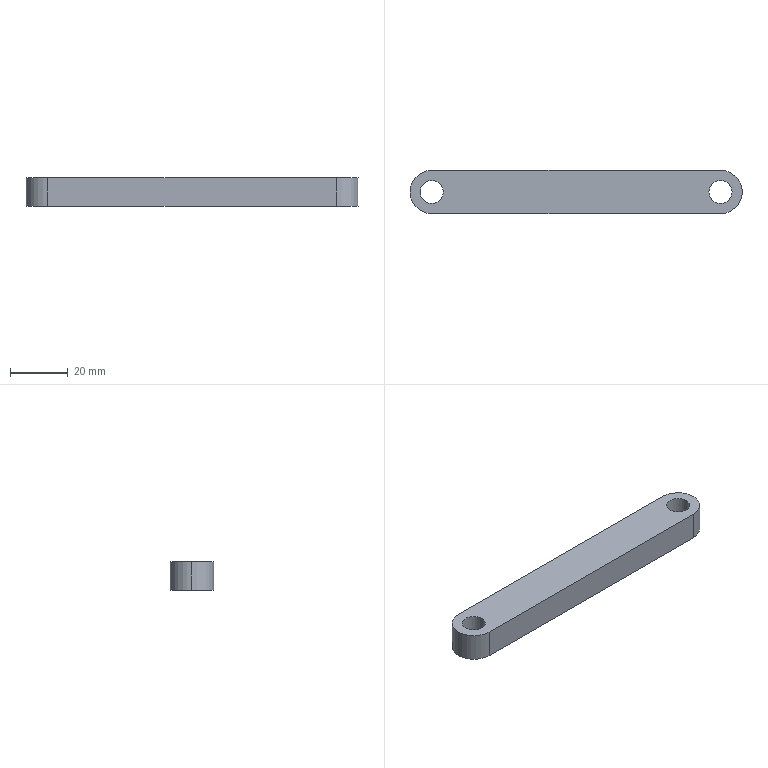Part | SolidWorks | features Extrusion 1 | 1 solid | 11 faces | box 115 x 15 x 10 mm | volume 15762 mm3 | cylinder 7 | plane 4 | commonest cylinder face diameters 8 x4 15 x3
STEP:
#1=CARTESIAN_POINT('',(96.,0.,10.));
#2=VERTEX_POINT('',#1);
#3=CARTESIAN_POINT('',(104.,0.,10.));
#4=VERTEX_POINT('',#3);
#5=CARTESIAN_POINT('',(100.,0.,10.));
#6=DIRECTION('',(0.,0.,1.));
#7=DIRECTION('',(1.,0.,0.));
#8=AXIS2_PLACEMENT_3D('',#5,#6,#7);
#9=CIRCLE('',#8,4.);
#10=EDGE_CURVE('',#2,#4,#9,.T.);
#11=ORIENTED_EDGE('',*,*,#10,.T.);
#12=CARTESIAN_POINT('',(104.,0.,0.));
#13=VERTEX_POINT('',#12);
#14=CARTESIAN_POINT('',(104.,0.,10.));
#15=DIRECTION('',(0.,0.,-1.));
#16=VECTOR('',#15,1000.);
#17=LINE('',#14,#16);
#18=EDGE_CURVE('',#4,#13,#17,.T.);
#19=ORIENTED_EDGE('',*,*,#18,.T.);
#20=CARTESIAN_POINT('',(96.,0.,0.));
#21=VERTEX_POINT('',#20);
#22=CARTESIAN_POINT('',(100.,0.,0.));
#23=DIRECTION('',(0.,0.,1.));
#24=DIRECTION('',(1.,0.,0.));
#25=AXIS2_PLACEMENT_3D('',#22,#23,#24);
#26=CIRCLE('',#25,4.);
#27=EDGE_CURVE('',#21,#13,#26,.T.);
#28=ORIENTED_EDGE('',*,*,#27,.F.);
#29=CARTESIAN_POINT('',(96.,0.,10.));
#30=DIRECTION('',(0.,0.,-1.));
#31=VECTOR('',#30,1000.);
#32=LINE('',#29,#31);
#33=EDGE_CURVE('',#2,#21,#32,.T.);
#34=ORIENTED_EDGE('',*,*,#33,.F.);
#35=EDGE_LOOP('',(#11,#19,#28,#34));
#36=FACE_OUTER_BOUND('',#35,.T.);
#37=CARTESIAN_POINT('',(100.,0.,10.));
#38=DIRECTION('',(0.,0.,-1.));
#39=DIRECTION('',(-1.,0.,0.));
#40=AXIS2_PLACEMENT_3D('',#37,#38,#39);
#41=CYLINDRICAL_SURFACE('',#40,4.);
#42=ADVANCED_FACE('',(#36),#41,.F.);
#43=CARTESIAN_POINT('',(-4.,0.,10.));
#44=VERTEX_POINT('',#43);
#45=CARTESIAN_POINT('',(4.,0.,10.));
#46=VERTEX_POINT('',#45);
#47=CARTESIAN_POINT('',(0.,0.,10.));
#48=DIRECTION('',(0.,0.,1.));
#49=DIRECTION('',(1.,0.,0.));
#50=AXIS2_PLACEMENT_3D('',#47,#48,#49);
#51=CIRCLE('',#50,4.);
#52=EDGE_CURVE('',#44,#46,#51,.T.);
#53=ORIENTED_EDGE('',*,*,#52,.T.);
#54=CARTESIAN_POINT('',(4.,0.,0.));
#55=VERTEX_POINT('',#54);
#56=CARTESIAN_POINT('',(4.,0.,10.));
#57=DIRECTION('',(0.,0.,-1.));
#58=VECTOR('',#57,1000.);
#59=LINE('',#56,#58);
#60=EDGE_CURVE('',#46,#55,#59,.T.);
#61=ORIENTED_EDGE('',*,*,#60,.T.);
#62=CARTESIAN_POINT('',(-4.,0.,0.));
#63=VERTEX_POINT('',#62);
#64=CARTESIAN_POINT('',(0.,0.,0.));
#65=DIRECTION('',(0.,0.,1.));
#66=DIRECTION('',(1.,0.,0.));
#67=AXIS2_PLACEMENT_3D('',#64,#65,#66);
#68=CIRCLE('',#67,4.);
#69=EDGE_CURVE('',#63,#55,#68,.T.);
#70=ORIENTED_EDGE('',*,*,#69,.F.);
#71=CARTESIAN_POINT('',(-4.,0.,10.));
#72=DIRECTION('',(0.,0.,-1.));
#73=VECTOR('',#72,1000.);
#74=LINE('',#71,#73);
#75=EDGE_CURVE('',#44,#63,#74,.T.);
#76=ORIENTED_EDGE('',*,*,#75,.F.);
#77=EDGE_LOOP('',(#53,#61,#70,#76));
#78=FACE_OUTER_BOUND('',#77,.T.);
#79=CARTESIAN_POINT('',(0.,0.,10.));
#80=DIRECTION('',(0.,0.,-1.));
#81=DIRECTION('',(-1.,0.,0.));
#82=AXIS2_PLACEMENT_3D('',#79,#80,#81);
#83=CYLINDRICAL_SURFACE('',#82,4.);
#84=ADVANCED_FACE('',(#78),#83,.F.);
#85=CARTESIAN_POINT('',(-7.5,0.,10.));
#86=VERTEX_POINT('',#85);
#87=CARTESIAN_POINT('',(0.,-7.5,10.));
#88=VERTEX_POINT('',#87);
#89=CARTESIAN_POINT('',(0.,0.,10.));
#90=DIRECTION('',(0.,0.,1.));
#91=DIRECTION('',(1.,0.,0.));
#92=AXIS2_PLACEMENT_3D('',#89,#90,#91);
#93=CIRCLE('',#92,7.5);
#94=EDGE_CURVE('',#86,#88,#93,.T.);
#95=ORIENTED_EDGE('',*,*,#94,.F.);
#96=CARTESIAN_POINT('',(-7.5,0.,0.));
#97=VERTEX_POINT('',#96);
#98=CARTESIAN_POINT('',(-7.5,0.,10.));
#99=DIRECTION('',(0.,0.,-1.));
#100=VECTOR('',#99,1000.);
#101=LINE('',#98,#100);
#102=EDGE_CURVE('',#86,#97,#101,.T.);
#103=ORIENTED_EDGE('',*,*,#102,.T.);
#104=CARTESIAN_POINT('',(0.,-7.5,0.));
#105=VERTEX_POINT('',#104);
#106=CARTESIAN_POINT('',(0.,0.,0.));
#107=DIRECTION('',(0.,0.,1.));
#108=DIRECTION('',(1.,0.,0.));
#109=AXIS2_PLACEMENT_3D('',#106,#107,#108);
#110=CIRCLE('',#109,7.5);
#111=EDGE_CURVE('',#97,#105,#110,.T.);
#112=ORIENTED_EDGE('',*,*,#111,.T.);
#113=CARTESIAN_POINT('',(0.,-7.5,10.));
#114=DIRECTION('',(0.,0.,-1.));
#115=VECTOR('',#114,1000.);
#116=LINE('',#113,#115);
#117=EDGE_CURVE('',#88,#105,#116,.T.);
#118=ORIENTED_EDGE('',*,*,#117,.F.);
#119=EDGE_LOOP('',(#95,#103,#112,#118));
#120=FACE_OUTER_BOUND('',#119,.T.);
#121=CARTESIAN_POINT('',(0.,0.,10.));
#122=DIRECTION('',(0.,0.,-1.));
#123=DIRECTION('',(-1.,0.,0.));
#124=AXIS2_PLACEMENT_3D('',#121,#122,#123);
#125=CYLINDRICAL_SURFACE('',#124,7.5);
#126=ADVANCED_FACE('',(#120),#125,.T.);
#127=ORIENTED_EDGE('',*,*,#52,.F.);
#128=CARTESIAN_POINT('',(0.,0.,10.));
#129=DIRECTION('',(0.,0.,1.));
#130=DIRECTION('',(1.,0.,0.));
#131=AXIS2_PLACEMENT_3D('',#128,#129,#130);
#132=CIRCLE('',#131,4.);
#133=EDGE_CURVE('',#46,#44,#132,.T.);
#134=ORIENTED_EDGE('',*,*,#133,.F.);
#135=EDGE_LOOP('',(#127,#134));
#136=FACE_BOUND('',#135,.T.);
#137=CARTESIAN_POINT('',(0.,7.5,10.));
#138=VERTEX_POINT('',#137);
#139=CARTESIAN_POINT('',(0.,0.,10.));
#140=DIRECTION('',(0.,0.,1.));
#141=DIRECTION('',(1.,0.,0.));
#142=AXIS2_PLACEMENT_3D('',#139,#140,#141);
#143=CIRCLE('',#142,7.5);
#144=EDGE_CURVE('',#138,#86,#143,.T.);
#145=ORIENTED_EDGE('',*,*,#144,.T.);
#146=ORIENTED_EDGE('',*,*,#94,.T.);
#147=CARTESIAN_POINT('',(100.,-7.5,10.));
#148=VERTEX_POINT('',#147);
#149=CARTESIAN_POINT('',(100.,-7.5,10.));
#150=DIRECTION('',(1.,0.,0.));
#151=VECTOR('',#150,1000.);
#152=LINE('',#149,#151);
#153=EDGE_CURVE('',#88,#148,#152,.T.);
#154=ORIENTED_EDGE('',*,*,#153,.T.);
#155=CARTESIAN_POINT('',(100.,7.5,10.));
#156=VERTEX_POINT('',#155);
#157=CARTESIAN_POINT('',(100.,0.,10.));
#158=DIRECTION('',(0.,0.,1.));
#159=DIRECTION('',(1.,0.,0.));
#160=AXIS2_PLACEMENT_3D('',#157,#158,#159);
#161=CIRCLE('',#160,7.5);
#162=EDGE_CURVE('',#148,#156,#161,.T.);
#163=ORIENTED_EDGE('',*,*,#162,.T.);
#164=CARTESIAN_POINT('',(0.,7.5,10.));
#165=DIRECTION('',(-1.,0.,0.));
#166=VECTOR('',#165,1000.);
#167=LINE('',#164,#166);
#168=EDGE_CURVE('',#156,#138,#167,.T.);
#169=ORIENTED_EDGE('',*,*,#168,.T.);
#170=EDGE_LOOP('',(#145,#146,#154,#163,#169));
#171=FACE_OUTER_BOUND('',#170,.T.);
#172=ORIENTED_EDGE('',*,*,#10,.F.);
#173=CARTESIAN_POINT('',(100.,0.,10.));
#174=DIRECTION('',(0.,0.,1.));
#175=DIRECTION('',(1.,0.,0.));
#176=AXIS2_PLACEMENT_3D('',#173,#174,#175);
#177=CIRCLE('',#176,4.);
#178=EDGE_CURVE('',#4,#2,#177,.T.);
#179=ORIENTED_EDGE('',*,*,#178,.F.);
#180=EDGE_LOOP('',(#172,#179));
#181=FACE_BOUND('',#180,.T.);
#182=CARTESIAN_POINT('',(0.,0.,10.));
#183=DIRECTION('',(0.,0.,1.));
#184=DIRECTION('',(1.,0.,0.));
#185=AXIS2_PLACEMENT_3D('',#182,#183,#184);
#186=PLANE('',#185);
#187=ADVANCED_FACE('',(#136,#171,#181),#186,.T.);
#188=CARTESIAN_POINT('',(0.,7.5,0.));
#189=VERTEX_POINT('',#188);
#190=CARTESIAN_POINT('',(0.,0.,0.));
#191=DIRECTION('',(0.,0.,1.));
#192=DIRECTION('',(1.,0.,0.));
#193=AXIS2_PLACEMENT_3D('',#190,#191,#192);
#194=CIRCLE('',#193,7.5);
#195=EDGE_CURVE('',#189,#97,#194,.T.);
#196=ORIENTED_EDGE('',*,*,#195,.F.);
#197=CARTESIAN_POINT('',(100.,7.5,0.));
#198=VERTEX_POINT('',#197);
#199=CARTESIAN_POINT('',(0.,7.5,0.));
#200=DIRECTION('',(-1.,0.,0.));
#201=VECTOR('',#200,1000.);
#202=LINE('',#199,#201);
#203=EDGE_CURVE('',#198,#189,#202,.T.);
#204=ORIENTED_EDGE('',*,*,#203,.F.);
#205=CARTESIAN_POINT('',(100.,-7.5,0.));
#206=VERTEX_POINT('',#205);
#207=CARTESIAN_POINT('',(100.,0.,0.));
#208=DIRECTION('',(0.,0.,1.));
#209=DIRECTION('',(1.,0.,0.));
#210=AXIS2_PLACEMENT_3D('',#207,#208,#209);
#211=CIRCLE('',#210,7.5);
#212=EDGE_CURVE('',#206,#198,#211,.T.);
#213=ORIENTED_EDGE('',*,*,#212,.F.);
#214=CARTESIAN_POINT('',(100.,-7.5,0.));
#215=DIRECTION('',(1.,0.,0.));
#216=VECTOR('',#215,1000.);
#217=LINE('',#214,#216);
#218=EDGE_CURVE('',#105,#206,#217,.T.);
#219=ORIENTED_EDGE('',*,*,#218,.F.);
#220=ORIENTED_EDGE('',*,*,#111,.F.);
#221=EDGE_LOOP('',(#196,#204,#213,#219,#220));
#222=FACE_OUTER_BOUND('',#221,.T.);
#223=ORIENTED_EDGE('',*,*,#69,.T.);
#224=CARTESIAN_POINT('',(0.,0.,0.));
#225=DIRECTION('',(0.,0.,1.));
#226=DIRECTION('',(1.,0.,0.));
#227=AXIS2_PLACEMENT_3D('',#224,#225,#226);
#228=CIRCLE('',#227,4.);
#229=EDGE_CURVE('',#55,#63,#228,.T.);
#230=ORIENTED_EDGE('',*,*,#229,.T.);
#231=EDGE_LOOP('',(#223,#230));
#232=FACE_BOUND('',#231,.T.);
#233=ORIENTED_EDGE('',*,*,#27,.T.);
#234=CARTESIAN_POINT('',(100.,0.,0.));
#235=DIRECTION('',(0.,0.,1.));
#236=DIRECTION('',(1.,0.,0.));
#237=AXIS2_PLACEMENT_3D('',#234,#235,#236);
#238=CIRCLE('',#237,4.);
#239=EDGE_CURVE('',#13,#21,#238,.T.);
#240=ORIENTED_EDGE('',*,*,#239,.T.);
#241=EDGE_LOOP('',(#233,#240));
#242=FACE_BOUND('',#241,.T.);
#243=CARTESIAN_POINT('',(0.,0.,0.));
#244=DIRECTION('',(0.,0.,1.));
#245=DIRECTION('',(1.,0.,0.));
#246=AXIS2_PLACEMENT_3D('',#243,#244,#245);
#247=PLANE('',#246);
#248=ADVANCED_FACE('',(#222,#232,#242),#247,.F.);
#249=ORIENTED_EDGE('',*,*,#102,.F.);
#250=ORIENTED_EDGE('',*,*,#144,.F.);
#251=CARTESIAN_POINT('',(0.,7.5,10.));
#252=DIRECTION('',(0.,0.,-1.));
#253=VECTOR('',#252,1000.);
#254=LINE('',#251,#253);
#255=EDGE_CURVE('',#138,#189,#254,.T.);
#256=ORIENTED_EDGE('',*,*,#255,.T.);
#257=ORIENTED_EDGE('',*,*,#195,.T.);
#258=EDGE_LOOP('',(#249,#250,#256,#257));
#259=FACE_OUTER_BOUND('',#258,.T.);
#260=CARTESIAN_POINT('',(0.,0.,10.));
#261=DIRECTION('',(0.,0.,-1.));
#262=DIRECTION('',(-1.,0.,0.));
#263=AXIS2_PLACEMENT_3D('',#260,#261,#262);
#264=CYLINDRICAL_SURFACE('',#263,7.5);
#265=ADVANCED_FACE('',(#259),#264,.T.);
#266=ORIENTED_EDGE('',*,*,#218,.T.);
#267=CARTESIAN_POINT('',(100.,-7.5,10.));
#268=DIRECTION('',(0.,0.,-1.));
#269=VECTOR('',#268,1000.);
#270=LINE('',#267,#269);
#271=EDGE_CURVE('',#148,#206,#270,.T.);
#272=ORIENTED_EDGE('',*,*,#271,.F.);
#273=ORIENTED_EDGE('',*,*,#153,.F.);
#274=ORIENTED_EDGE('',*,*,#117,.T.);
#275=EDGE_LOOP('',(#266,#272,#273,#274));
#276=FACE_OUTER_BOUND('',#275,.T.);
#277=CARTESIAN_POINT('',(100.,-7.5,10.));
#278=DIRECTION('',(0.,1.,0.));
#279=DIRECTION('',(-1.,0.,0.));
#280=AXIS2_PLACEMENT_3D('',#277,#278,#279);
#281=PLANE('',#280);
#282=ADVANCED_FACE('',(#276),#281,.F.);
#283=ORIENTED_EDGE('',*,*,#212,.T.);
#284=CARTESIAN_POINT('',(100.,7.5,10.));
#285=DIRECTION('',(0.,0.,-1.));
#286=VECTOR('',#285,1000.);
#287=LINE('',#284,#286);
#288=EDGE_CURVE('',#156,#198,#287,.T.);
#289=ORIENTED_EDGE('',*,*,#288,.F.);
#290=ORIENTED_EDGE('',*,*,#162,.F.);
#291=ORIENTED_EDGE('',*,*,#271,.T.);
#292=EDGE_LOOP('',(#283,#289,#290,#291));
#293=FACE_OUTER_BOUND('',#292,.T.);
#294=CARTESIAN_POINT('',(100.,0.,10.));
#295=DIRECTION('',(0.,0.,-1.));
#296=DIRECTION('',(-1.,0.,0.));
#297=AXIS2_PLACEMENT_3D('',#294,#295,#296);
#298=CYLINDRICAL_SURFACE('',#297,7.5);
#299=ADVANCED_FACE('',(#293),#298,.T.);
#300=ORIENTED_EDGE('',*,*,#203,.T.);
#301=ORIENTED_EDGE('',*,*,#255,.F.);
#302=ORIENTED_EDGE('',*,*,#168,.F.);
#303=ORIENTED_EDGE('',*,*,#288,.T.);
#304=EDGE_LOOP('',(#300,#301,#302,#303));
#305=FACE_OUTER_BOUND('',#304,.T.);
#306=CARTESIAN_POINT('',(0.,7.5,10.));
#307=DIRECTION('',(0.,-1.,0.));
#308=DIRECTION('',(1.,0.,0.));
#309=AXIS2_PLACEMENT_3D('',#306,#307,#308);
#310=PLANE('',#309);
#311=ADVANCED_FACE('',(#305),#310,.F.);
#312=ORIENTED_EDGE('',*,*,#60,.F.);
#313=ORIENTED_EDGE('',*,*,#133,.T.);
#314=ORIENTED_EDGE('',*,*,#75,.T.);
#315=ORIENTED_EDGE('',*,*,#229,.F.);
#316=EDGE_LOOP('',(#312,#313,#314,#315));
#317=FACE_OUTER_BOUND('',#316,.T.);
#318=CARTESIAN_POINT('',(0.,0.,10.));
#319=DIRECTION('',(0.,0.,-1.));
#320=DIRECTION('',(-1.,0.,0.));
#321=AXIS2_PLACEMENT_3D('',#318,#319,#320);
#322=CYLINDRICAL_SURFACE('',#321,4.);
#323=ADVANCED_FACE('',(#317),#322,.F.);
#324=ORIENTED_EDGE('',*,*,#18,.F.);
#325=ORIENTED_EDGE('',*,*,#178,.T.);
#326=ORIENTED_EDGE('',*,*,#33,.T.);
#327=ORIENTED_EDGE('',*,*,#239,.F.);
#328=EDGE_LOOP('',(#324,#325,#326,#327));
#329=FACE_OUTER_BOUND('',#328,.T.);
#330=CARTESIAN_POINT('',(100.,0.,10.));
#331=DIRECTION('',(0.,0.,-1.));
#332=DIRECTION('',(-1.,0.,0.));
#333=AXIS2_PLACEMENT_3D('',#330,#331,#332);
#334=CYLINDRICAL_SURFACE('',#333,4.);
#335=ADVANCED_FACE('',(#329),#334,.F.);
#336=CLOSED_SHELL('',(#42,#84,#126,#187,#248,#265,#282,#299,#311,#323,#335));
#337=MANIFOLD_SOLID_BREP('',#336);
#338=CARTESIAN_POINT('',(0.,0.,0.));
#339=DIRECTION('',(0.,0.,1.));
#340=DIRECTION('',(1.,0.,0.));
#341=AXIS2_PLACEMENT_3D('',#338,#339,#340);
#342=(LENGTH_UNIT()NAMED_UNIT(*)SI_UNIT(.MILLI.,.METRE.));
#343=UNCERTAINTY_MEASURE_WITH_UNIT(LENGTH_MEASURE(0.00001),#342,'','');
#344=(NAMED_UNIT(*)PLANE_ANGLE_UNIT()SI_UNIT($,.RADIAN.));
#345=(NAMED_UNIT(*)SI_UNIT($,.STERADIAN.)SOLID_ANGLE_UNIT());
#346=(GEOMETRIC_REPRESENTATION_CONTEXT(3)GLOBAL_UNCERTAINTY_ASSIGNED_CONTEXT((#343))GLOBAL_UNIT_ASSIGNED_CONTEXT((#342,#344,#345))REPRESENTATION_CONTEXT('',''));
#347=ADVANCED_BREP_SHAPE_REPRESENTATION('',(#337,#341),#346);